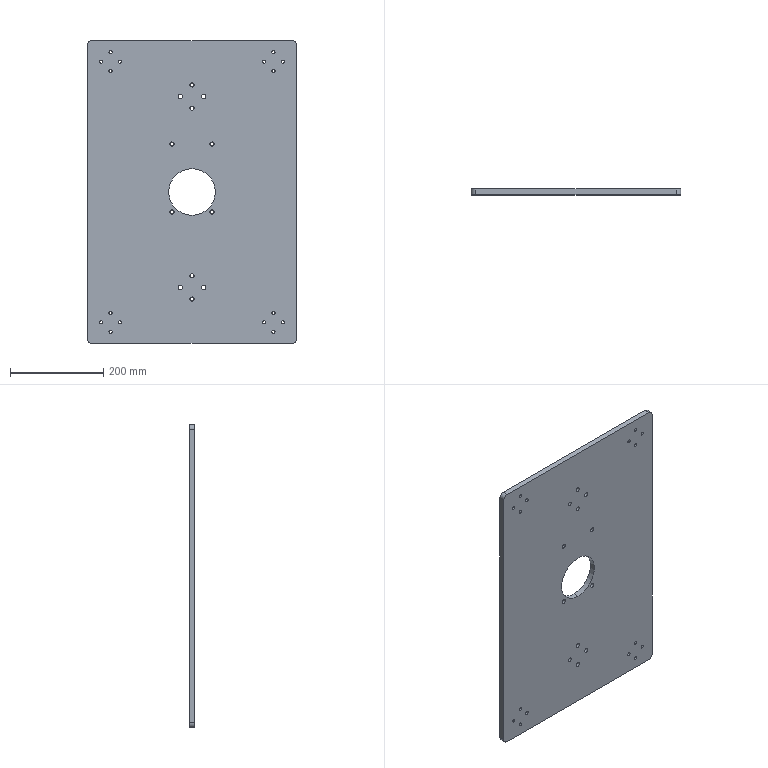Part | SolidWorks | features BaseBody 1 | 1 solid | 68 faces | box 450 x 12 x 650 mm | volume 3398172 mm3 | cylinder 62 | plane 6 | commonest cylinder face diameters 7 x32 9 x24 20 x4 100 x2